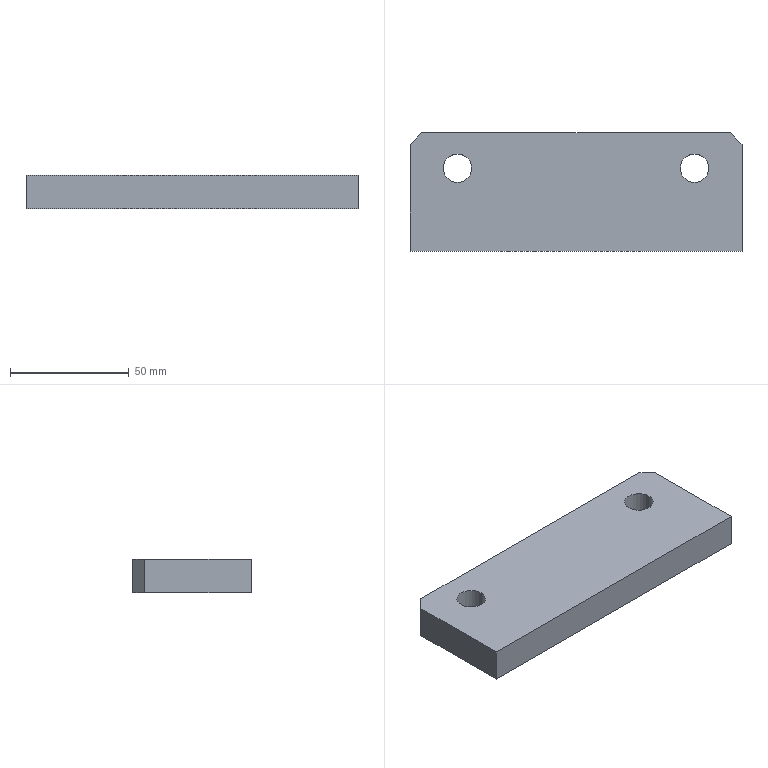Part | STEP file | [02]-2 | 1 solid | 12 faces | box 140 x 50 x 14 mm | volume 94483 mm3 | plane 8 | cylinder 4 | commonest cylinder face diameters 12 x4
STEP:
#1=CARTESIAN_POINT('',(126.,35.,14.));
#2=VERTEX_POINT('',#1);
#3=CARTESIAN_POINT('',(114.,35.,14.));
#4=VERTEX_POINT('',#3);
#5=CARTESIAN_POINT('',(120.,35.,14.));
#6=DIRECTION('',(0.,0.,1.));
#7=DIRECTION('',(1.,0.,0.));
#8=AXIS2_PLACEMENT_3D('',#5,#6,#7);
#9=CIRCLE('',#8,6.);
#10=EDGE_CURVE('',#2,#4,#9,.T.);
#11=ORIENTED_EDGE('',*,*,#10,.T.);
#12=CARTESIAN_POINT('',(114.,35.,0.));
#13=VERTEX_POINT('',#12);
#14=CARTESIAN_POINT('',(114.,35.,14.));
#15=DIRECTION('',(0.,0.,-1.));
#16=VECTOR('',#15,1000.);
#17=LINE('',#14,#16);
#18=EDGE_CURVE('',#4,#13,#17,.T.);
#19=ORIENTED_EDGE('',*,*,#18,.T.);
#20=CARTESIAN_POINT('',(126.,35.,0.));
#21=VERTEX_POINT('',#20);
#22=CARTESIAN_POINT('',(120.,35.,0.));
#23=DIRECTION('',(0.,0.,-1.));
#24=DIRECTION('',(-1.,0.,0.));
#25=AXIS2_PLACEMENT_3D('',#22,#23,#24);
#26=CIRCLE('',#25,6.);
#27=EDGE_CURVE('',#13,#21,#26,.T.);
#28=ORIENTED_EDGE('',*,*,#27,.T.);
#29=CARTESIAN_POINT('',(126.,35.,14.));
#30=DIRECTION('',(0.,0.,-1.));
#31=VECTOR('',#30,1000.);
#32=LINE('',#29,#31);
#33=EDGE_CURVE('',#2,#21,#32,.T.);
#34=ORIENTED_EDGE('',*,*,#33,.F.);
#35=EDGE_LOOP('',(#11,#19,#28,#34));
#36=FACE_OUTER_BOUND('',#35,.T.);
#37=CARTESIAN_POINT('',(120.,35.,14.));
#38=DIRECTION('',(0.,0.,-1.));
#39=DIRECTION('',(1.,0.,0.));
#40=AXIS2_PLACEMENT_3D('',#37,#38,#39);
#41=CYLINDRICAL_SURFACE('',#40,6.);
#42=ADVANCED_FACE('',(#36),#41,.F.);
#43=CARTESIAN_POINT('',(26.,35.,14.));
#44=VERTEX_POINT('',#43);
#45=CARTESIAN_POINT('',(14.,35.,14.));
#46=VERTEX_POINT('',#45);
#47=CARTESIAN_POINT('',(20.,35.,14.));
#48=DIRECTION('',(0.,0.,1.));
#49=DIRECTION('',(1.,0.,0.));
#50=AXIS2_PLACEMENT_3D('',#47,#48,#49);
#51=CIRCLE('',#50,6.);
#52=EDGE_CURVE('',#44,#46,#51,.T.);
#53=ORIENTED_EDGE('',*,*,#52,.T.);
#54=CARTESIAN_POINT('',(14.,35.,0.));
#55=VERTEX_POINT('',#54);
#56=CARTESIAN_POINT('',(14.,35.,14.));
#57=DIRECTION('',(0.,0.,-1.));
#58=VECTOR('',#57,1000.);
#59=LINE('',#56,#58);
#60=EDGE_CURVE('',#46,#55,#59,.T.);
#61=ORIENTED_EDGE('',*,*,#60,.T.);
#62=CARTESIAN_POINT('',(26.,35.,0.));
#63=VERTEX_POINT('',#62);
#64=CARTESIAN_POINT('',(20.,35.,0.));
#65=DIRECTION('',(0.,0.,-1.));
#66=DIRECTION('',(-1.,0.,0.));
#67=AXIS2_PLACEMENT_3D('',#64,#65,#66);
#68=CIRCLE('',#67,6.);
#69=EDGE_CURVE('',#55,#63,#68,.T.);
#70=ORIENTED_EDGE('',*,*,#69,.T.);
#71=CARTESIAN_POINT('',(26.,35.,14.));
#72=DIRECTION('',(0.,0.,-1.));
#73=VECTOR('',#72,1000.);
#74=LINE('',#71,#73);
#75=EDGE_CURVE('',#44,#63,#74,.T.);
#76=ORIENTED_EDGE('',*,*,#75,.F.);
#77=EDGE_LOOP('',(#53,#61,#70,#76));
#78=FACE_OUTER_BOUND('',#77,.T.);
#79=CARTESIAN_POINT('',(20.,35.,14.));
#80=DIRECTION('',(0.,0.,-1.));
#81=DIRECTION('',(1.,0.,0.));
#82=AXIS2_PLACEMENT_3D('',#79,#80,#81);
#83=CYLINDRICAL_SURFACE('',#82,6.);
#84=ADVANCED_FACE('',(#78),#83,.F.);
#85=ORIENTED_EDGE('',*,*,#10,.F.);
#86=CARTESIAN_POINT('',(120.,35.,14.));
#87=DIRECTION('',(0.,0.,1.));
#88=DIRECTION('',(1.,0.,0.));
#89=AXIS2_PLACEMENT_3D('',#86,#87,#88);
#90=CIRCLE('',#89,6.);
#91=EDGE_CURVE('',#4,#2,#90,.T.);
#92=ORIENTED_EDGE('',*,*,#91,.F.);
#93=EDGE_LOOP('',(#85,#92));
#94=FACE_BOUND('',#93,.T.);
#95=ORIENTED_EDGE('',*,*,#52,.F.);
#96=CARTESIAN_POINT('',(20.,35.,14.));
#97=DIRECTION('',(0.,0.,1.));
#98=DIRECTION('',(1.,0.,0.));
#99=AXIS2_PLACEMENT_3D('',#96,#97,#98);
#100=CIRCLE('',#99,6.);
#101=EDGE_CURVE('',#46,#44,#100,.T.);
#102=ORIENTED_EDGE('',*,*,#101,.F.);
#103=EDGE_LOOP('',(#95,#102));
#104=FACE_BOUND('',#103,.T.);
#105=CARTESIAN_POINT('',(135.,50.,14.));
#106=VERTEX_POINT('',#105);
#107=CARTESIAN_POINT('',(5.,50.,14.));
#108=VERTEX_POINT('',#107);
#109=CARTESIAN_POINT('',(70.,50.,14.));
#110=DIRECTION('',(-1.,0.,0.));
#111=VECTOR('',#110,1000.);
#112=LINE('',#109,#111);
#113=EDGE_CURVE('',#106,#108,#112,.T.);
#114=ORIENTED_EDGE('',*,*,#113,.T.);
#115=CARTESIAN_POINT('',(0.,45.,14.));
#116=VERTEX_POINT('',#115);
#117=CARTESIAN_POINT('',(25.,70.,14.));
#118=DIRECTION('',(0.7071,0.7071,0.));
#119=VECTOR('',#118,1000.);
#120=LINE('',#117,#119);
#121=EDGE_CURVE('',#116,#108,#120,.T.);
#122=ORIENTED_EDGE('',*,*,#121,.F.);
#123=CARTESIAN_POINT('',(0.,0.,14.));
#124=VERTEX_POINT('',#123);
#125=CARTESIAN_POINT('',(0.,25.,14.));
#126=DIRECTION('',(0.,-1.,0.));
#127=VECTOR('',#126,1000.);
#128=LINE('',#125,#127);
#129=EDGE_CURVE('',#116,#124,#128,.T.);
#130=ORIENTED_EDGE('',*,*,#129,.T.);
#131=CARTESIAN_POINT('',(140.,0.,14.));
#132=VERTEX_POINT('',#131);
#133=CARTESIAN_POINT('',(70.,0.,14.));
#134=DIRECTION('',(1.,0.,0.));
#135=VECTOR('',#134,1000.);
#136=LINE('',#133,#135);
#137=EDGE_CURVE('',#124,#132,#136,.T.);
#138=ORIENTED_EDGE('',*,*,#137,.T.);
#139=CARTESIAN_POINT('',(140.,45.,14.));
#140=VERTEX_POINT('',#139);
#141=CARTESIAN_POINT('',(140.,25.,14.));
#142=DIRECTION('',(0.,1.,0.));
#143=VECTOR('',#142,1000.);
#144=LINE('',#141,#143);
#145=EDGE_CURVE('',#132,#140,#144,.T.);
#146=ORIENTED_EDGE('',*,*,#145,.T.);
#147=CARTESIAN_POINT('',(115.,70.,14.));
#148=DIRECTION('',(0.7071,-0.7071,0.));
#149=VECTOR('',#148,1000.);
#150=LINE('',#147,#149);
#151=EDGE_CURVE('',#106,#140,#150,.T.);
#152=ORIENTED_EDGE('',*,*,#151,.F.);
#153=EDGE_LOOP('',(#114,#122,#130,#138,#146,#152));
#154=FACE_OUTER_BOUND('',#153,.T.);
#155=CARTESIAN_POINT('',(70.,25.,14.));
#156=DIRECTION('',(0.,0.,1.));
#157=DIRECTION('',(-1.,0.,0.));
#158=AXIS2_PLACEMENT_3D('',#155,#156,#157);
#159=PLANE('',#158);
#160=ADVANCED_FACE('',(#94,#104,#154),#159,.T.);
#161=CARTESIAN_POINT('',(0.,0.,0.));
#162=VERTEX_POINT('',#161);
#163=CARTESIAN_POINT('',(0.,0.,0.));
#164=DIRECTION('',(0.,0.,1.));
#165=VECTOR('',#164,1000.);
#166=LINE('',#163,#165);
#167=EDGE_CURVE('',#162,#124,#166,.T.);
#168=ORIENTED_EDGE('',*,*,#167,.F.);
#169=CARTESIAN_POINT('',(140.,0.,0.));
#170=VERTEX_POINT('',#169);
#171=CARTESIAN_POINT('',(70.,0.,0.));
#172=DIRECTION('',(-1.,0.,0.));
#173=VECTOR('',#172,1000.);
#174=LINE('',#171,#173);
#175=EDGE_CURVE('',#170,#162,#174,.T.);
#176=ORIENTED_EDGE('',*,*,#175,.F.);
#177=CARTESIAN_POINT('',(140.,0.,0.));
#178=DIRECTION('',(0.,0.,1.));
#179=VECTOR('',#178,1000.);
#180=LINE('',#177,#179);
#181=EDGE_CURVE('',#170,#132,#180,.T.);
#182=ORIENTED_EDGE('',*,*,#181,.T.);
#183=ORIENTED_EDGE('',*,*,#137,.F.);
#184=EDGE_LOOP('',(#168,#176,#182,#183));
#185=FACE_OUTER_BOUND('',#184,.T.);
#186=CARTESIAN_POINT('',(70.,0.,0.));
#187=DIRECTION('',(0.,-1.,0.));
#188=DIRECTION('',(0.,0.,-1.));
#189=AXIS2_PLACEMENT_3D('',#186,#187,#188);
#190=PLANE('',#189);
#191=ADVANCED_FACE('',(#185),#190,.T.);
#192=ORIENTED_EDGE('',*,*,#145,.F.);
#193=ORIENTED_EDGE('',*,*,#181,.F.);
#194=CARTESIAN_POINT('',(140.,45.,0.));
#195=VERTEX_POINT('',#194);
#196=CARTESIAN_POINT('',(140.,25.,0.));
#197=DIRECTION('',(0.,-1.,0.));
#198=VECTOR('',#197,1000.);
#199=LINE('',#196,#198);
#200=EDGE_CURVE('',#195,#170,#199,.T.);
#201=ORIENTED_EDGE('',*,*,#200,.F.);
#202=CARTESIAN_POINT('',(140.,45.,0.));
#203=DIRECTION('',(0.,0.,-1.));
#204=VECTOR('',#203,1000.);
#205=LINE('',#202,#204);
#206=EDGE_CURVE('',#140,#195,#205,.T.);
#207=ORIENTED_EDGE('',*,*,#206,.F.);
#208=EDGE_LOOP('',(#192,#193,#201,#207));
#209=FACE_OUTER_BOUND('',#208,.T.);
#210=CARTESIAN_POINT('',(140.,25.,0.));
#211=DIRECTION('',(1.,0.,0.));
#212=DIRECTION('',(0.,0.,1.));
#213=AXIS2_PLACEMENT_3D('',#210,#211,#212);
#214=PLANE('',#213);
#215=ADVANCED_FACE('',(#209),#214,.T.);
#216=CARTESIAN_POINT('',(5.,50.,0.));
#217=VERTEX_POINT('',#216);
#218=CARTESIAN_POINT('',(135.,50.,0.));
#219=VERTEX_POINT('',#218);
#220=CARTESIAN_POINT('',(70.,50.,0.));
#221=DIRECTION('',(1.,0.,0.));
#222=VECTOR('',#221,1000.);
#223=LINE('',#220,#222);
#224=EDGE_CURVE('',#217,#219,#223,.T.);
#225=ORIENTED_EDGE('',*,*,#224,.F.);
#226=CARTESIAN_POINT('',(5.,50.,0.));
#227=DIRECTION('',(0.,0.,-1.));
#228=VECTOR('',#227,1000.);
#229=LINE('',#226,#228);
#230=EDGE_CURVE('',#108,#217,#229,.T.);
#231=ORIENTED_EDGE('',*,*,#230,.F.);
#232=ORIENTED_EDGE('',*,*,#113,.F.);
#233=CARTESIAN_POINT('',(135.,50.,0.));
#234=DIRECTION('',(0.,0.,1.));
#235=VECTOR('',#234,1000.);
#236=LINE('',#233,#235);
#237=EDGE_CURVE('',#219,#106,#236,.T.);
#238=ORIENTED_EDGE('',*,*,#237,.F.);
#239=EDGE_LOOP('',(#225,#231,#232,#238));
#240=FACE_OUTER_BOUND('',#239,.T.);
#241=CARTESIAN_POINT('',(70.,50.,0.));
#242=DIRECTION('',(0.,1.,0.));
#243=DIRECTION('',(0.,0.,1.));
#244=AXIS2_PLACEMENT_3D('',#241,#242,#243);
#245=PLANE('',#244);
#246=ADVANCED_FACE('',(#240),#245,.T.);
#247=CARTESIAN_POINT('',(120.,35.,0.));
#248=DIRECTION('',(0.,0.,-1.));
#249=DIRECTION('',(-1.,0.,0.));
#250=AXIS2_PLACEMENT_3D('',#247,#248,#249);
#251=CIRCLE('',#250,6.);
#252=EDGE_CURVE('',#21,#13,#251,.T.);
#253=ORIENTED_EDGE('',*,*,#252,.F.);
#254=ORIENTED_EDGE('',*,*,#27,.F.);
#255=EDGE_LOOP('',(#253,#254));
#256=FACE_BOUND('',#255,.T.);
#257=CARTESIAN_POINT('',(20.,35.,0.));
#258=DIRECTION('',(0.,0.,-1.));
#259=DIRECTION('',(-1.,0.,0.));
#260=AXIS2_PLACEMENT_3D('',#257,#258,#259);
#261=CIRCLE('',#260,6.);
#262=EDGE_CURVE('',#63,#55,#261,.T.);
#263=ORIENTED_EDGE('',*,*,#262,.F.);
#264=ORIENTED_EDGE('',*,*,#69,.F.);
#265=EDGE_LOOP('',(#263,#264));
#266=FACE_BOUND('',#265,.T.);
#267=ORIENTED_EDGE('',*,*,#200,.T.);
#268=ORIENTED_EDGE('',*,*,#175,.T.);
#269=CARTESIAN_POINT('',(0.,45.,0.));
#270=VERTEX_POINT('',#269);
#271=CARTESIAN_POINT('',(0.,25.,0.));
#272=DIRECTION('',(0.,1.,0.));
#273=VECTOR('',#272,1000.);
#274=LINE('',#271,#273);
#275=EDGE_CURVE('',#162,#270,#274,.T.);
#276=ORIENTED_EDGE('',*,*,#275,.T.);
#277=CARTESIAN_POINT('',(25.,70.,0.));
#278=DIRECTION('',(-0.7071,-0.7071,0.));
#279=VECTOR('',#278,1000.);
#280=LINE('',#277,#279);
#281=EDGE_CURVE('',#217,#270,#280,.T.);
#282=ORIENTED_EDGE('',*,*,#281,.F.);
#283=ORIENTED_EDGE('',*,*,#224,.T.);
#284=CARTESIAN_POINT('',(115.,70.,0.));
#285=DIRECTION('',(-0.7071,0.7071,0.));
#286=VECTOR('',#285,1000.);
#287=LINE('',#284,#286);
#288=EDGE_CURVE('',#195,#219,#287,.T.);
#289=ORIENTED_EDGE('',*,*,#288,.F.);
#290=EDGE_LOOP('',(#267,#268,#276,#282,#283,#289));
#291=FACE_OUTER_BOUND('',#290,.T.);
#292=CARTESIAN_POINT('',(70.,25.,0.));
#293=DIRECTION('',(0.,0.,-1.));
#294=DIRECTION('',(1.,0.,0.));
#295=AXIS2_PLACEMENT_3D('',#292,#293,#294);
#296=PLANE('',#295);
#297=ADVANCED_FACE('',(#256,#266,#291),#296,.T.);
#298=ORIENTED_EDGE('',*,*,#275,.F.);
#299=ORIENTED_EDGE('',*,*,#167,.T.);
#300=ORIENTED_EDGE('',*,*,#129,.F.);
#301=CARTESIAN_POINT('',(0.,45.,0.));
#302=DIRECTION('',(0.,0.,1.));
#303=VECTOR('',#302,1000.);
#304=LINE('',#301,#303);
#305=EDGE_CURVE('',#270,#116,#304,.T.);
#306=ORIENTED_EDGE('',*,*,#305,.F.);
#307=EDGE_LOOP('',(#298,#299,#300,#306));
#308=FACE_OUTER_BOUND('',#307,.T.);
#309=CARTESIAN_POINT('',(0.,25.,0.));
#310=DIRECTION('',(-1.,0.,0.));
#311=DIRECTION('',(0.,0.,-1.));
#312=AXIS2_PLACEMENT_3D('',#309,#310,#311);
#313=PLANE('',#312);
#314=ADVANCED_FACE('',(#308),#313,.T.);
#315=ORIENTED_EDGE('',*,*,#288,.T.);
#316=ORIENTED_EDGE('',*,*,#237,.T.);
#317=ORIENTED_EDGE('',*,*,#151,.T.);
#318=ORIENTED_EDGE('',*,*,#206,.T.);
#319=EDGE_LOOP('',(#315,#316,#317,#318));
#320=FACE_OUTER_BOUND('',#319,.T.);
#321=CARTESIAN_POINT('',(135.,50.,0.));
#322=DIRECTION('',(-0.7071,-0.7071,0.));
#323=DIRECTION('',(0.,0.,1.));
#324=AXIS2_PLACEMENT_3D('',#321,#322,#323);
#325=PLANE('',#324);
#326=ADVANCED_FACE('',(#320),#325,.F.);
#327=ORIENTED_EDGE('',*,*,#281,.T.);
#328=ORIENTED_EDGE('',*,*,#305,.T.);
#329=ORIENTED_EDGE('',*,*,#121,.T.);
#330=ORIENTED_EDGE('',*,*,#230,.T.);
#331=EDGE_LOOP('',(#327,#328,#329,#330));
#332=FACE_OUTER_BOUND('',#331,.T.);
#333=CARTESIAN_POINT('',(0.,45.,0.));
#334=DIRECTION('',(0.7071,-0.7071,0.));
#335=DIRECTION('',(0.,0.,1.));
#336=AXIS2_PLACEMENT_3D('',#333,#334,#335);
#337=PLANE('',#336);
#338=ADVANCED_FACE('',(#332),#337,.F.);
#339=ORIENTED_EDGE('',*,*,#60,.F.);
#340=ORIENTED_EDGE('',*,*,#101,.T.);
#341=ORIENTED_EDGE('',*,*,#75,.T.);
#342=ORIENTED_EDGE('',*,*,#262,.T.);
#343=EDGE_LOOP('',(#339,#340,#341,#342));
#344=FACE_OUTER_BOUND('',#343,.T.);
#345=CARTESIAN_POINT('',(20.,35.,14.));
#346=DIRECTION('',(0.,0.,-1.));
#347=DIRECTION('',(1.,0.,0.));
#348=AXIS2_PLACEMENT_3D('',#345,#346,#347);
#349=CYLINDRICAL_SURFACE('',#348,6.);
#350=ADVANCED_FACE('',(#344),#349,.F.);
#351=ORIENTED_EDGE('',*,*,#18,.F.);
#352=ORIENTED_EDGE('',*,*,#91,.T.);
#353=ORIENTED_EDGE('',*,*,#33,.T.);
#354=ORIENTED_EDGE('',*,*,#252,.T.);
#355=EDGE_LOOP('',(#351,#352,#353,#354));
#356=FACE_OUTER_BOUND('',#355,.T.);
#357=CARTESIAN_POINT('',(120.,35.,14.));
#358=DIRECTION('',(0.,0.,-1.));
#359=DIRECTION('',(1.,0.,0.));
#360=AXIS2_PLACEMENT_3D('',#357,#358,#359);
#361=CYLINDRICAL_SURFACE('',#360,6.);
#362=ADVANCED_FACE('',(#356),#361,.F.);
#363=CLOSED_SHELL('',(#42,#84,#160,#191,#215,#246,#297,#314,#326,#338,#350,#362));
#364=MANIFOLD_SOLID_BREP('',#363);
#365=CARTESIAN_POINT('',(0.,0.,0.));
#366=DIRECTION('',(0.,0.,1.));
#367=DIRECTION('',(1.,0.,0.));
#368=AXIS2_PLACEMENT_3D('',#365,#366,#367);
#369=(LENGTH_UNIT()NAMED_UNIT(*)SI_UNIT(.MILLI.,.METRE.));
#370=UNCERTAINTY_MEASURE_WITH_UNIT(LENGTH_MEASURE(0.00001),#369,'','');
#371=(NAMED_UNIT(*)PLANE_ANGLE_UNIT()SI_UNIT($,.RADIAN.));
#372=(NAMED_UNIT(*)SI_UNIT($,.STERADIAN.)SOLID_ANGLE_UNIT());
#373=(GEOMETRIC_REPRESENTATION_CONTEXT(3)GLOBAL_UNCERTAINTY_ASSIGNED_CONTEXT((#370))GLOBAL_UNIT_ASSIGNED_CONTEXT((#369,#371,#372))REPRESENTATION_CONTEXT('',''));
#374=ADVANCED_BREP_SHAPE_REPRESENTATION('',(#364,#368),#373);